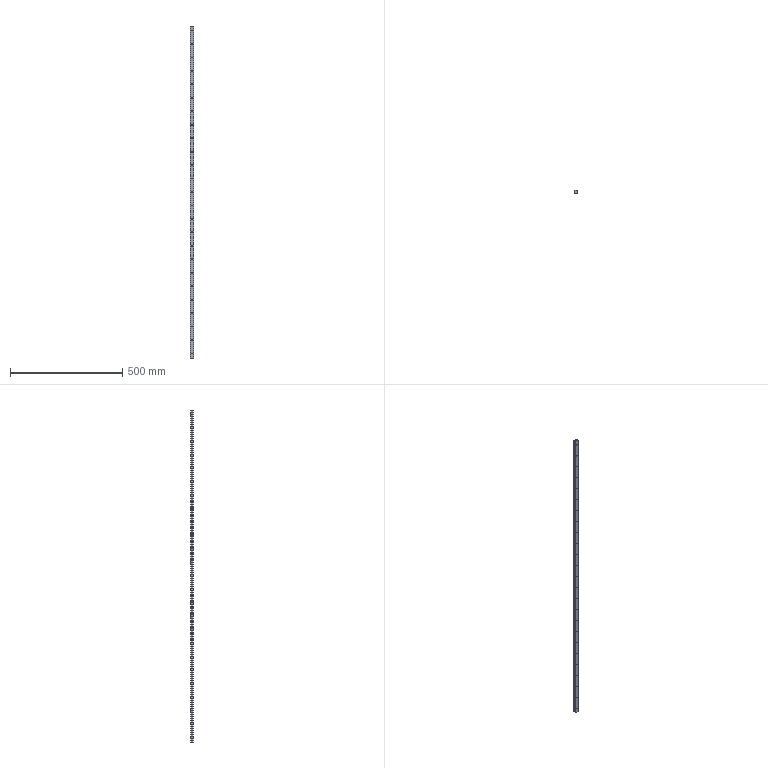Part | STEP file | 0245_Z_018_SX2WT24-1480_1 | 1 solid | 142 faces | box 15 x 12.5 x 1480 mm | volume 246310 mm3 | cylinder 105 | plane 37 | commonest cylinder face diameters 3.5 x50 6 x50 4.4 x3 3 x2